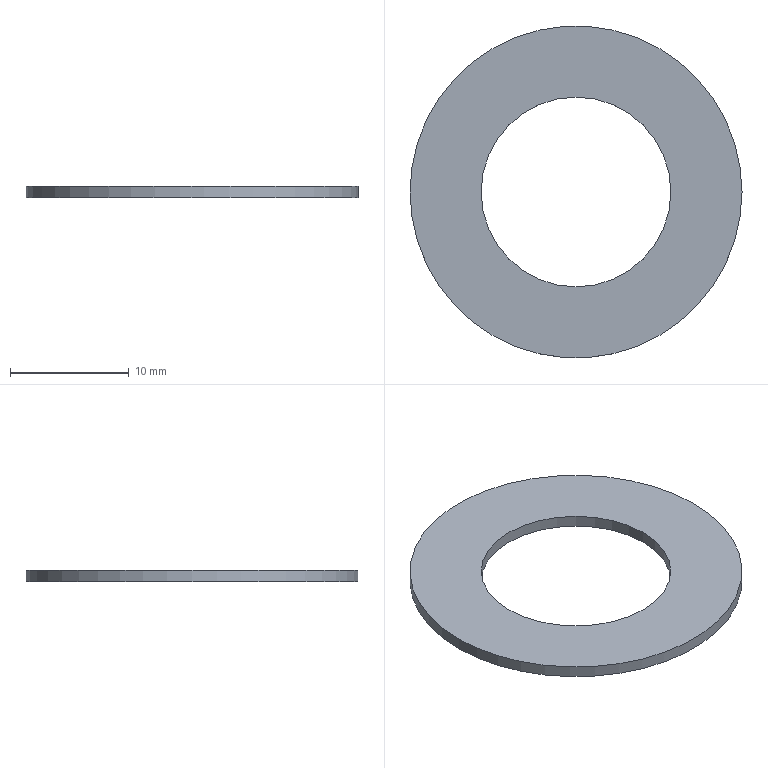Part | NX | features DATUM_CSYS 2, EXTRUDE 1, SKETCH 1 | 1 solid | 4 faces | box 28 x 28 x 1 mm | volume 414.69 mm3 | cylinder 2 | plane 2 | commonest cylinder face diameters 16 x1 28 x1
STEP:
#1=CARTESIAN_POINT('',(14.,0.,1.));
#2=VERTEX_POINT('',#1);
#3=CARTESIAN_POINT('',(0.,0.,1.));
#4=DIRECTION('',(0.,0.,-1.));
#5=DIRECTION('',(1.,0.,0.));
#6=AXIS2_PLACEMENT_3D('',#3,#4,#5);
#7=CIRCLE('',#6,14.);
#8=EDGE_CURVE('',#2,#2,#7,.T.);
#9=ORIENTED_EDGE('',*,*,#8,.T.);
#10=EDGE_LOOP('',(#9));
#11=FACE_BOUND('',#10,.T.);
#12=CARTESIAN_POINT('',(14.,0.,0.));
#13=VERTEX_POINT('',#12);
#14=CARTESIAN_POINT('',(0.,0.,0.));
#15=DIRECTION('',(0.,0.,-1.));
#16=DIRECTION('',(1.,0.,0.));
#17=AXIS2_PLACEMENT_3D('',#14,#15,#16);
#18=CIRCLE('',#17,14.);
#19=EDGE_CURVE('',#13,#13,#18,.T.);
#20=ORIENTED_EDGE('',*,*,#19,.F.);
#21=EDGE_LOOP('',(#20));
#22=FACE_BOUND('',#21,.T.);
#23=CARTESIAN_POINT('',(0.,0.,1.));
#24=DIRECTION('',(0.,0.,-1.));
#25=DIRECTION('',(-1.,0.,0.));
#26=AXIS2_PLACEMENT_3D('',#23,#24,#25);
#27=CYLINDRICAL_SURFACE('',#26,14.);
#28=ADVANCED_FACE('',(#11,#22),#27,.T.);
#29=CARTESIAN_POINT('',(8.,0.,1.));
#30=VERTEX_POINT('',#29);
#31=CARTESIAN_POINT('',(0.,0.,1.));
#32=DIRECTION('',(0.,0.,-1.));
#33=DIRECTION('',(1.,0.,0.));
#34=AXIS2_PLACEMENT_3D('',#31,#32,#33);
#35=CIRCLE('',#34,8.);
#36=EDGE_CURVE('',#30,#30,#35,.T.);
#37=ORIENTED_EDGE('',*,*,#36,.F.);
#38=EDGE_LOOP('',(#37));
#39=FACE_BOUND('',#38,.T.);
#40=CARTESIAN_POINT('',(8.,0.,0.));
#41=VERTEX_POINT('',#40);
#42=CARTESIAN_POINT('',(0.,0.,0.));
#43=DIRECTION('',(0.,0.,-1.));
#44=DIRECTION('',(1.,0.,0.));
#45=AXIS2_PLACEMENT_3D('',#42,#43,#44);
#46=CIRCLE('',#45,8.);
#47=EDGE_CURVE('',#41,#41,#46,.T.);
#48=ORIENTED_EDGE('',*,*,#47,.T.);
#49=EDGE_LOOP('',(#48));
#50=FACE_BOUND('',#49,.T.);
#51=CARTESIAN_POINT('',(0.,0.,1.));
#52=DIRECTION('',(0.,0.,-1.));
#53=DIRECTION('',(-1.,0.,0.));
#54=AXIS2_PLACEMENT_3D('',#51,#52,#53);
#55=CYLINDRICAL_SURFACE('',#54,8.);
#56=ADVANCED_FACE('',(#39,#50),#55,.F.);
#57=ORIENTED_EDGE('',*,*,#8,.F.);
#58=EDGE_LOOP('',(#57));
#59=FACE_BOUND('',#58,.T.);
#60=ORIENTED_EDGE('',*,*,#36,.T.);
#61=EDGE_LOOP('',(#60));
#62=FACE_BOUND('',#61,.T.);
#63=CARTESIAN_POINT('',(0.,0.,1.));
#64=DIRECTION('',(0.,0.,-1.));
#65=DIRECTION('',(-1.,0.,0.));
#66=AXIS2_PLACEMENT_3D('',#63,#64,#65);
#67=PLANE('',#66);
#68=ADVANCED_FACE('',(#59,#62),#67,.F.);
#69=ORIENTED_EDGE('',*,*,#19,.T.);
#70=EDGE_LOOP('',(#69));
#71=FACE_BOUND('',#70,.T.);
#72=ORIENTED_EDGE('',*,*,#47,.F.);
#73=EDGE_LOOP('',(#72));
#74=FACE_BOUND('',#73,.T.);
#75=CARTESIAN_POINT('',(0.,0.,0.));
#76=DIRECTION('',(0.,0.,-1.));
#77=DIRECTION('',(-1.,0.,0.));
#78=AXIS2_PLACEMENT_3D('',#75,#76,#77);
#79=PLANE('',#78);
#80=ADVANCED_FACE('',(#71,#74),#79,.T.);
#81=CLOSED_SHELL('',(#28,#56,#68,#80));
#82=MANIFOLD_SOLID_BREP('',#81);
#83=(LENGTH_UNIT()NAMED_UNIT(*)SI_UNIT(.MILLI.,.METRE.));
#84=UNCERTAINTY_MEASURE_WITH_UNIT(LENGTH_MEASURE(0.00001),#83,'','');
#85=(NAMED_UNIT(*)PLANE_ANGLE_UNIT()SI_UNIT($,.RADIAN.));
#86=(NAMED_UNIT(*)SI_UNIT($,.STERADIAN.)SOLID_ANGLE_UNIT());
#87=(GEOMETRIC_REPRESENTATION_CONTEXT(3)GLOBAL_UNCERTAINTY_ASSIGNED_CONTEXT((#84))GLOBAL_UNIT_ASSIGNED_CONTEXT((#83,#85,#86))REPRESENTATION_CONTEXT('',''));
#88=ADVANCED_BREP_SHAPE_REPRESENTATION('',(#82),#87);